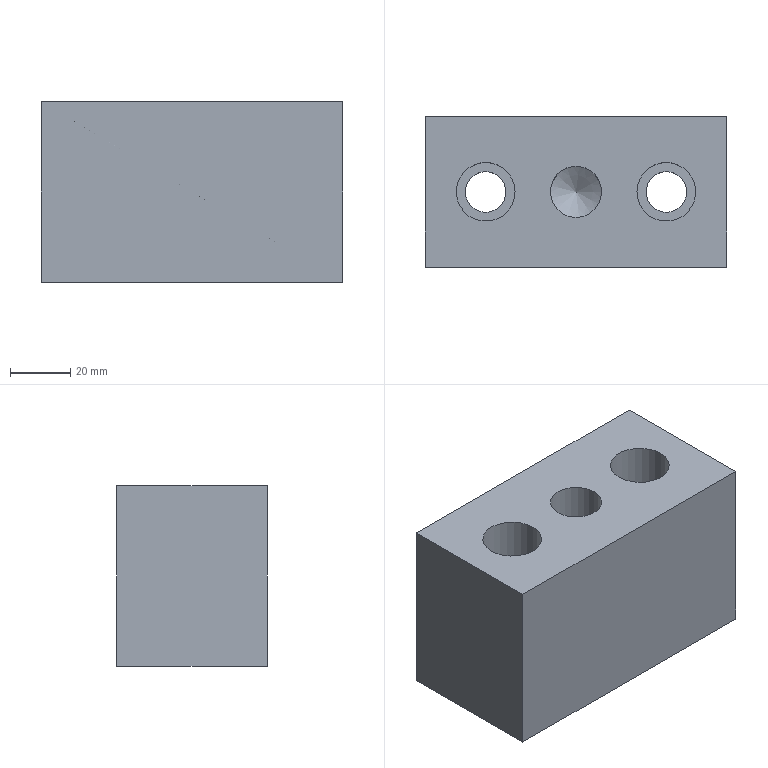Part | NX | features solid 2 | 1 solid | 14 faces | box 100 x 50 x 60 mm | volume 270962 mm3 | plane 8 | cylinder 5 | cone 1 | commonest cylinder face diameters 13.5 x2 19.5 x2 17 x1
STEP:
#1=CARTESIAN_POINT('',(-710.,420.,-30.));
#2=VERTEX_POINT('',#1);
#3=CARTESIAN_POINT('',(-610.,420.,-30.));
#4=VERTEX_POINT('',#3);
#5=CARTESIAN_POINT('',(-710.,420.,-30.));
#6=DIRECTION('',(-1.,0.,0.));
#7=VECTOR('',#6,1000.);
#8=LINE('',#5,#7);
#9=EDGE_CURVE('',#2,#4,#8,.F.);
#10=ORIENTED_EDGE('',*,*,#9,.F.);
#11=CARTESIAN_POINT('',(-710.,420.,30.));
#12=VERTEX_POINT('',#11);
#13=CARTESIAN_POINT('',(-710.,420.,30.));
#14=DIRECTION('',(0.,0.,-1.));
#15=VECTOR('',#14,1000.);
#16=LINE('',#13,#15);
#17=EDGE_CURVE('',#12,#2,#16,.T.);
#18=ORIENTED_EDGE('',*,*,#17,.F.);
#19=CARTESIAN_POINT('',(-610.,420.,30.));
#20=VERTEX_POINT('',#19);
#21=CARTESIAN_POINT('',(-710.,420.,30.));
#22=DIRECTION('',(-1.,0.,0.));
#23=VECTOR('',#22,1000.);
#24=LINE('',#21,#23);
#25=EDGE_CURVE('',#12,#20,#24,.F.);
#26=ORIENTED_EDGE('',*,*,#25,.T.);
#27=CARTESIAN_POINT('',(-610.,420.,30.));
#28=DIRECTION('',(0.,0.,-1.));
#29=VECTOR('',#28,1000.);
#30=LINE('',#27,#29);
#31=EDGE_CURVE('',#20,#4,#30,.T.);
#32=ORIENTED_EDGE('',*,*,#31,.T.);
#33=EDGE_LOOP('',(#10,#18,#26,#32));
#34=FACE_BOUND('',#33,.T.);
#35=CARTESIAN_POINT('',(-710.,420.,30.));
#36=DIRECTION('',(0.,-1.,0.));
#37=DIRECTION('',(0.,0.,1.));
#38=AXIS2_PLACEMENT_3D('',#35,#36,#37);
#39=PLANE('',#38);
#40=ADVANCED_FACE('',(#34),#39,.F.);
#41=CARTESIAN_POINT('',(-610.,370.,-30.));
#42=VERTEX_POINT('',#41);
#43=CARTESIAN_POINT('',(-610.,370.,-30.));
#44=DIRECTION('',(0.,1.,0.));
#45=VECTOR('',#44,1000.);
#46=LINE('',#43,#45);
#47=EDGE_CURVE('',#42,#4,#46,.T.);
#48=ORIENTED_EDGE('',*,*,#47,.T.);
#49=ORIENTED_EDGE('',*,*,#31,.F.);
#50=CARTESIAN_POINT('',(-610.,370.,30.));
#51=VERTEX_POINT('',#50);
#52=CARTESIAN_POINT('',(-610.,370.,30.));
#53=DIRECTION('',(0.,1.,0.));
#54=VECTOR('',#53,1000.);
#55=LINE('',#52,#54);
#56=EDGE_CURVE('',#51,#20,#55,.T.);
#57=ORIENTED_EDGE('',*,*,#56,.F.);
#58=CARTESIAN_POINT('',(-610.,370.,30.));
#59=DIRECTION('',(0.,0.,-1.));
#60=VECTOR('',#59,1000.);
#61=LINE('',#58,#60);
#62=EDGE_CURVE('',#51,#42,#61,.T.);
#63=ORIENTED_EDGE('',*,*,#62,.T.);
#64=EDGE_LOOP('',(#48,#49,#57,#63));
#65=FACE_BOUND('',#64,.T.);
#66=CARTESIAN_POINT('',(-610.,370.,30.));
#67=DIRECTION('',(1.,0.,0.));
#68=DIRECTION('',(0.,0.,-1.));
#69=AXIS2_PLACEMENT_3D('',#66,#67,#68);
#70=PLANE('',#69);
#71=ADVANCED_FACE('',(#65),#70,.T.);
#72=CARTESIAN_POINT('',(-710.,370.,-30.));
#73=VERTEX_POINT('',#72);
#74=CARTESIAN_POINT('',(-710.,370.,-30.));
#75=DIRECTION('',(-1.,0.,0.));
#76=VECTOR('',#75,1000.);
#77=LINE('',#74,#76);
#78=EDGE_CURVE('',#73,#42,#77,.F.);
#79=ORIENTED_EDGE('',*,*,#78,.T.);
#80=ORIENTED_EDGE('',*,*,#62,.F.);
#81=CARTESIAN_POINT('',(-710.,370.,30.));
#82=VERTEX_POINT('',#81);
#83=CARTESIAN_POINT('',(-710.,370.,30.));
#84=DIRECTION('',(-1.,0.,0.));
#85=VECTOR('',#84,1000.);
#86=LINE('',#83,#85);
#87=EDGE_CURVE('',#82,#51,#86,.F.);
#88=ORIENTED_EDGE('',*,*,#87,.F.);
#89=CARTESIAN_POINT('',(-710.,370.,30.));
#90=DIRECTION('',(0.,0.,-1.));
#91=VECTOR('',#90,1000.);
#92=LINE('',#89,#91);
#93=EDGE_CURVE('',#82,#73,#92,.T.);
#94=ORIENTED_EDGE('',*,*,#93,.T.);
#95=EDGE_LOOP('',(#79,#80,#88,#94));
#96=FACE_BOUND('',#95,.T.);
#97=CARTESIAN_POINT('',(-710.,370.,30.));
#98=DIRECTION('',(0.,-1.,0.));
#99=DIRECTION('',(0.,0.,1.));
#100=AXIS2_PLACEMENT_3D('',#97,#98,#99);
#101=PLANE('',#100);
#102=ADVANCED_FACE('',(#96),#101,.T.);
#103=CARTESIAN_POINT('',(-710.,370.,-30.));
#104=DIRECTION('',(0.,1.,0.));
#105=VECTOR('',#104,1000.);
#106=LINE('',#103,#105);
#107=EDGE_CURVE('',#73,#2,#106,.T.);
#108=ORIENTED_EDGE('',*,*,#107,.F.);
#109=ORIENTED_EDGE('',*,*,#93,.F.);
#110=CARTESIAN_POINT('',(-710.,370.,30.));
#111=DIRECTION('',(0.,1.,0.));
#112=VECTOR('',#111,1000.);
#113=LINE('',#110,#112);
#114=EDGE_CURVE('',#82,#12,#113,.T.);
#115=ORIENTED_EDGE('',*,*,#114,.T.);
#116=ORIENTED_EDGE('',*,*,#17,.T.);
#117=EDGE_LOOP('',(#108,#109,#115,#116));
#118=FACE_BOUND('',#117,.T.);
#119=CARTESIAN_POINT('',(-710.,370.,30.));
#120=DIRECTION('',(1.,0.,0.));
#121=DIRECTION('',(0.,0.,-1.));
#122=AXIS2_PLACEMENT_3D('',#119,#120,#121);
#123=PLANE('',#122);
#124=ADVANCED_FACE('',(#118),#123,.F.);
#125=CARTESIAN_POINT('',(-668.5,395.,30.));
#126=VERTEX_POINT('',#125);
#127=CARTESIAN_POINT('',(-660.,395.,30.));
#128=DIRECTION('',(0.,0.,1.));
#129=DIRECTION('',(-1.,0.,0.));
#130=AXIS2_PLACEMENT_3D('',#127,#128,#129);
#131=CIRCLE('',#130,8.5);
#132=EDGE_CURVE('',#126,#126,#131,.T.);
#133=ORIENTED_EDGE('',*,*,#132,.F.);
#134=EDGE_LOOP('',(#133));
#135=FACE_BOUND('',#134,.T.);
#136=CARTESIAN_POINT('',(-639.75,395.,30.));
#137=VERTEX_POINT('',#136);
#138=CARTESIAN_POINT('',(-630.,395.,30.));
#139=DIRECTION('',(0.,0.,1.));
#140=DIRECTION('',(-1.,0.,0.));
#141=AXIS2_PLACEMENT_3D('',#138,#139,#140);
#142=CIRCLE('',#141,9.75);
#143=EDGE_CURVE('',#137,#137,#142,.T.);
#144=ORIENTED_EDGE('',*,*,#143,.F.);
#145=EDGE_LOOP('',(#144));
#146=FACE_BOUND('',#145,.T.);
#147=CARTESIAN_POINT('',(-699.75,395.,30.));
#148=VERTEX_POINT('',#147);
#149=CARTESIAN_POINT('',(-690.,395.,30.));
#150=DIRECTION('',(0.,0.,1.));
#151=DIRECTION('',(-1.,0.,0.));
#152=AXIS2_PLACEMENT_3D('',#149,#150,#151);
#153=CIRCLE('',#152,9.75);
#154=EDGE_CURVE('',#148,#148,#153,.T.);
#155=ORIENTED_EDGE('',*,*,#154,.F.);
#156=EDGE_LOOP('',(#155));
#157=FACE_BOUND('',#156,.T.);
#158=ORIENTED_EDGE('',*,*,#25,.F.);
#159=ORIENTED_EDGE('',*,*,#114,.F.);
#160=ORIENTED_EDGE('',*,*,#87,.T.);
#161=ORIENTED_EDGE('',*,*,#56,.T.);
#162=EDGE_LOOP('',(#158,#159,#160,#161));
#163=FACE_BOUND('',#162,.T.);
#164=CARTESIAN_POINT('',(-710.,370.,30.));
#165=DIRECTION('',(0.,0.,-1.));
#166=DIRECTION('',(0.,1.,0.));
#167=AXIS2_PLACEMENT_3D('',#164,#165,#166);
#168=PLANE('',#167);
#169=ADVANCED_FACE('',(#135,#146,#157,#163),#168,.F.);
#170=CARTESIAN_POINT('',(-636.75,395.,-30.));
#171=VERTEX_POINT('',#170);
#172=CARTESIAN_POINT('',(-630.,395.,-30.));
#173=DIRECTION('',(0.,0.,1.));
#174=DIRECTION('',(-1.,0.,0.));
#175=AXIS2_PLACEMENT_3D('',#172,#173,#174);
#176=CIRCLE('',#175,6.75);
#177=EDGE_CURVE('',#171,#171,#176,.T.);
#178=ORIENTED_EDGE('',*,*,#177,.T.);
#179=EDGE_LOOP('',(#178));
#180=FACE_BOUND('',#179,.T.);
#181=CARTESIAN_POINT('',(-696.75,395.,-30.));
#182=VERTEX_POINT('',#181);
#183=CARTESIAN_POINT('',(-690.,395.,-30.));
#184=DIRECTION('',(0.,0.,1.));
#185=DIRECTION('',(-1.,0.,0.));
#186=AXIS2_PLACEMENT_3D('',#183,#184,#185);
#187=CIRCLE('',#186,6.75);
#188=EDGE_CURVE('',#182,#182,#187,.T.);
#189=ORIENTED_EDGE('',*,*,#188,.T.);
#190=EDGE_LOOP('',(#189));
#191=FACE_BOUND('',#190,.T.);
#192=ORIENTED_EDGE('',*,*,#9,.T.);
#193=ORIENTED_EDGE('',*,*,#47,.F.);
#194=ORIENTED_EDGE('',*,*,#78,.F.);
#195=ORIENTED_EDGE('',*,*,#107,.T.);
#196=EDGE_LOOP('',(#192,#193,#194,#195));
#197=FACE_BOUND('',#196,.T.);
#198=CARTESIAN_POINT('',(-710.,370.,-30.));
#199=DIRECTION('',(0.,0.,-1.));
#200=DIRECTION('',(0.,1.,0.));
#201=AXIS2_PLACEMENT_3D('',#198,#199,#200);
#202=PLANE('',#201);
#203=ADVANCED_FACE('',(#180,#191,#197),#202,.T.);
#204=ORIENTED_EDGE('',*,*,#188,.F.);
#205=EDGE_LOOP('',(#204));
#206=FACE_BOUND('',#205,.T.);
#207=CARTESIAN_POINT('',(-696.75,395.,15.));
#208=VERTEX_POINT('',#207);
#209=CARTESIAN_POINT('',(-690.,395.,15.));
#210=DIRECTION('',(0.,0.,1.));
#211=DIRECTION('',(-1.,0.,0.));
#212=AXIS2_PLACEMENT_3D('',#209,#210,#211);
#213=CIRCLE('',#212,6.75);
#214=EDGE_CURVE('',#208,#208,#213,.T.);
#215=ORIENTED_EDGE('',*,*,#214,.T.);
#216=EDGE_LOOP('',(#215));
#217=FACE_BOUND('',#216,.T.);
#218=CARTESIAN_POINT('',(-690.,395.,-30.));
#219=DIRECTION('',(0.,0.,-1.));
#220=DIRECTION('',(-1.,0.,0.));
#221=AXIS2_PLACEMENT_3D('',#218,#219,#220);
#222=CYLINDRICAL_SURFACE('',#221,6.75);
#223=ADVANCED_FACE('',(#206,#217),#222,.F.);
#224=ORIENTED_EDGE('',*,*,#214,.F.);
#225=EDGE_LOOP('',(#224));
#226=FACE_BOUND('',#225,.T.);
#227=CARTESIAN_POINT('',(-699.75,395.,15.));
#228=VERTEX_POINT('',#227);
#229=CARTESIAN_POINT('',(-690.,395.,15.));
#230=DIRECTION('',(0.,0.,1.));
#231=DIRECTION('',(-1.,0.,0.));
#232=AXIS2_PLACEMENT_3D('',#229,#230,#231);
#233=CIRCLE('',#232,9.75);
#234=EDGE_CURVE('',#228,#228,#233,.T.);
#235=ORIENTED_EDGE('',*,*,#234,.T.);
#236=EDGE_LOOP('',(#235));
#237=FACE_BOUND('',#236,.T.);
#238=CARTESIAN_POINT('',(-690.,395.,15.));
#239=DIRECTION('',(0.,0.,-1.));
#240=DIRECTION('',(-1.,0.,0.));
#241=AXIS2_PLACEMENT_3D('',#238,#239,#240);
#242=PLANE('',#241);
#243=ADVANCED_FACE('',(#226,#237),#242,.F.);
#244=ORIENTED_EDGE('',*,*,#234,.F.);
#245=EDGE_LOOP('',(#244));
#246=FACE_BOUND('',#245,.T.);
#247=ORIENTED_EDGE('',*,*,#154,.T.);
#248=EDGE_LOOP('',(#247));
#249=FACE_BOUND('',#248,.T.);
#250=CARTESIAN_POINT('',(-690.,395.,30.));
#251=DIRECTION('',(0.,0.,-1.));
#252=DIRECTION('',(-1.,0.,0.));
#253=AXIS2_PLACEMENT_3D('',#250,#251,#252);
#254=CYLINDRICAL_SURFACE('',#253,9.75);
#255=ADVANCED_FACE('',(#246,#249),#254,.F.);
#256=ORIENTED_EDGE('',*,*,#177,.F.);
#257=EDGE_LOOP('',(#256));
#258=FACE_BOUND('',#257,.T.);
#259=CARTESIAN_POINT('',(-636.75,395.,15.));
#260=VERTEX_POINT('',#259);
#261=CARTESIAN_POINT('',(-630.,395.,15.));
#262=DIRECTION('',(0.,0.,1.));
#263=DIRECTION('',(-1.,0.,0.));
#264=AXIS2_PLACEMENT_3D('',#261,#262,#263);
#265=CIRCLE('',#264,6.75);
#266=EDGE_CURVE('',#260,#260,#265,.T.);
#267=ORIENTED_EDGE('',*,*,#266,.T.);
#268=EDGE_LOOP('',(#267));
#269=FACE_BOUND('',#268,.T.);
#270=CARTESIAN_POINT('',(-630.,395.,-30.));
#271=DIRECTION('',(0.,0.,-1.));
#272=DIRECTION('',(-1.,0.,0.));
#273=AXIS2_PLACEMENT_3D('',#270,#271,#272);
#274=CYLINDRICAL_SURFACE('',#273,6.75);
#275=ADVANCED_FACE('',(#258,#269),#274,.F.);
#276=ORIENTED_EDGE('',*,*,#266,.F.);
#277=EDGE_LOOP('',(#276));
#278=FACE_BOUND('',#277,.T.);
#279=CARTESIAN_POINT('',(-639.75,395.,15.));
#280=VERTEX_POINT('',#279);
#281=CARTESIAN_POINT('',(-630.,395.,15.));
#282=DIRECTION('',(0.,0.,1.));
#283=DIRECTION('',(-1.,0.,0.));
#284=AXIS2_PLACEMENT_3D('',#281,#282,#283);
#285=CIRCLE('',#284,9.75);
#286=EDGE_CURVE('',#280,#280,#285,.T.);
#287=ORIENTED_EDGE('',*,*,#286,.T.);
#288=EDGE_LOOP('',(#287));
#289=FACE_BOUND('',#288,.T.);
#290=CARTESIAN_POINT('',(-630.,395.,15.));
#291=DIRECTION('',(0.,0.,-1.));
#292=DIRECTION('',(-1.,0.,0.));
#293=AXIS2_PLACEMENT_3D('',#290,#291,#292);
#294=PLANE('',#293);
#295=ADVANCED_FACE('',(#278,#289),#294,.F.);
#296=ORIENTED_EDGE('',*,*,#286,.F.);
#297=EDGE_LOOP('',(#296));
#298=FACE_BOUND('',#297,.T.);
#299=ORIENTED_EDGE('',*,*,#143,.T.);
#300=EDGE_LOOP('',(#299));
#301=FACE_BOUND('',#300,.T.);
#302=CARTESIAN_POINT('',(-630.,395.,30.));
#303=DIRECTION('',(0.,0.,-1.));
#304=DIRECTION('',(-1.,0.,0.));
#305=AXIS2_PLACEMENT_3D('',#302,#303,#304);
#306=CYLINDRICAL_SURFACE('',#305,9.75);
#307=ADVANCED_FACE('',(#298,#301),#306,.F.);
#308=ORIENTED_EDGE('',*,*,#132,.T.);
#309=EDGE_LOOP('',(#308));
#310=FACE_BOUND('',#309,.T.);
#311=CARTESIAN_POINT('',(-668.5,395.,0.));
#312=VERTEX_POINT('',#311);
#313=CARTESIAN_POINT('',(-660.,395.,0.));
#314=DIRECTION('',(0.,0.,1.));
#315=DIRECTION('',(-1.,0.,0.));
#316=AXIS2_PLACEMENT_3D('',#313,#314,#315);
#317=CIRCLE('',#316,8.5);
#318=EDGE_CURVE('',#312,#312,#317,.T.);
#319=ORIENTED_EDGE('',*,*,#318,.F.);
#320=EDGE_LOOP('',(#319));
#321=FACE_BOUND('',#320,.T.);
#322=CARTESIAN_POINT('',(-660.,395.,30.));
#323=DIRECTION('',(0.,0.,-1.));
#324=DIRECTION('',(-1.,0.,0.));
#325=AXIS2_PLACEMENT_3D('',#322,#323,#324);
#326=CYLINDRICAL_SURFACE('',#325,8.5);
#327=ADVANCED_FACE('',(#310,#321),#326,.F.);
#328=ORIENTED_EDGE('',*,*,#318,.T.);
#329=EDGE_LOOP('',(#328));
#330=FACE_BOUND('',#329,.T.);
#331=CARTESIAN_POINT('',(-660.,395.,-5.107));
#332=VERTEX_POINT('',#331);
#333=VERTEX_LOOP('',#332);
#334=FACE_BOUND('',#333,.T.);
#335=CARTESIAN_POINT('',(-660.,395.,0.));
#336=DIRECTION('',(0.,0.,1.));
#337=DIRECTION('',(1.,0.,0.));
#338=AXIS2_PLACEMENT_3D('',#335,#336,#337);
#339=CONICAL_SURFACE('',#338,8.5,1.03);
#340=ADVANCED_FACE('',(#330,#334),#339,.F.);
#341=CLOSED_SHELL('',(#40,#71,#102,#124,#169,#203,#223,#243,#255,#275,#295,#307,#327,#340));
#342=MANIFOLD_SOLID_BREP('',#341);
#343=(LENGTH_UNIT()NAMED_UNIT(*)SI_UNIT(.MILLI.,.METRE.));
#344=UNCERTAINTY_MEASURE_WITH_UNIT(LENGTH_MEASURE(0.00001),#343,'','');
#345=(NAMED_UNIT(*)PLANE_ANGLE_UNIT()SI_UNIT($,.RADIAN.));
#346=(NAMED_UNIT(*)SI_UNIT($,.STERADIAN.)SOLID_ANGLE_UNIT());
#347=(GEOMETRIC_REPRESENTATION_CONTEXT(3)GLOBAL_UNCERTAINTY_ASSIGNED_CONTEXT((#344))GLOBAL_UNIT_ASSIGNED_CONTEXT((#343,#345,#346))REPRESENTATION_CONTEXT('',''));
#348=ADVANCED_BREP_SHAPE_REPRESENTATION('',(#342),#347);